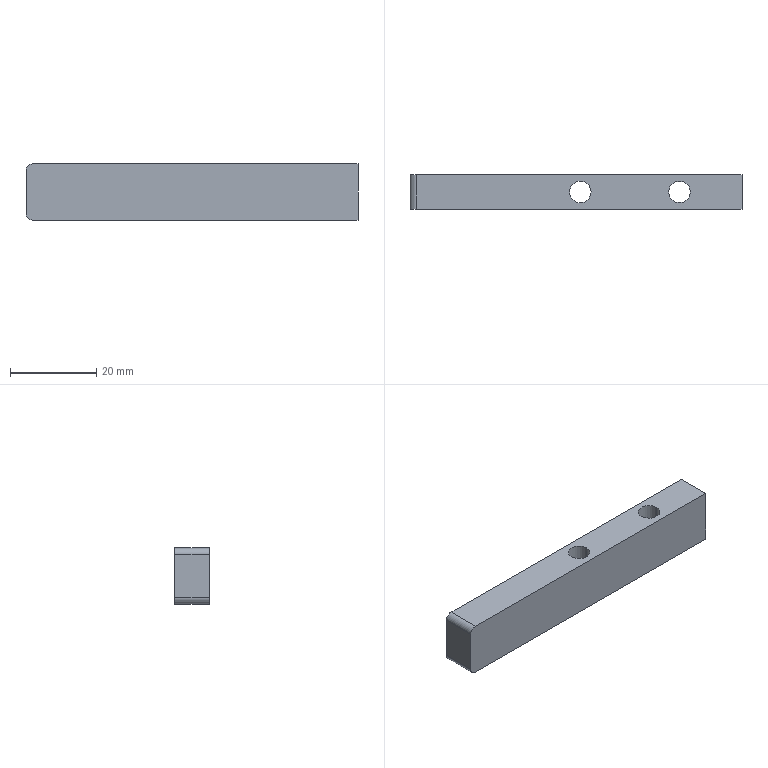Part | 1 solid | 15 faces | box 77 x 8 x 13 mm | volume 6967 mm3 | cylinder 8 | plane 7 | commonest cylinder face diameters 5 x4 3 x2 11 x2
STEP:
#1=CARTESIAN_POINT('',(-14.,4.,-6.5));
#2=VERTEX_POINT('',#1);
#3=CARTESIAN_POINT('',(-9.,4.,-6.5));
#4=VERTEX_POINT('',#3);
#5=CARTESIAN_POINT('',(-11.5,4.,-6.5));
#6=DIRECTION('',(0.,0.,1.));
#7=DIRECTION('',(1.,0.,0.));
#8=AXIS2_PLACEMENT_3D('',#5,#6,#7);
#9=CIRCLE('',#8,2.5);
#10=EDGE_CURVE('',#2,#4,#9,.T.);
#11=ORIENTED_EDGE('',*,*,#10,.F.);
#12=CARTESIAN_POINT('',(-14.,4.,6.5));
#13=VERTEX_POINT('',#12);
#14=CARTESIAN_POINT('',(-14.,4.,-6.5));
#15=DIRECTION('',(0.,0.,1.));
#16=VECTOR('',#15,1000.);
#17=LINE('',#14,#16);
#18=EDGE_CURVE('',#2,#13,#17,.T.);
#19=ORIENTED_EDGE('',*,*,#18,.T.);
#20=CARTESIAN_POINT('',(-9.,4.,6.5));
#21=VERTEX_POINT('',#20);
#22=CARTESIAN_POINT('',(-11.5,4.,6.5));
#23=DIRECTION('',(0.,0.,1.));
#24=DIRECTION('',(1.,0.,0.));
#25=AXIS2_PLACEMENT_3D('',#22,#23,#24);
#26=CIRCLE('',#25,2.5);
#27=EDGE_CURVE('',#13,#21,#26,.T.);
#28=ORIENTED_EDGE('',*,*,#27,.T.);
#29=CARTESIAN_POINT('',(-9.,4.,-6.5));
#30=DIRECTION('',(0.,0.,1.));
#31=VECTOR('',#30,1000.);
#32=LINE('',#29,#31);
#33=EDGE_CURVE('',#4,#21,#32,.T.);
#34=ORIENTED_EDGE('',*,*,#33,.F.);
#35=EDGE_LOOP('',(#11,#19,#28,#34));
#36=FACE_OUTER_BOUND('',#35,.T.);
#37=CARTESIAN_POINT('',(-11.5,4.,-6.5));
#38=DIRECTION('',(0.,0.,1.));
#39=DIRECTION('',(1.,0.,0.));
#40=AXIS2_PLACEMENT_3D('',#37,#38,#39);
#41=CYLINDRICAL_SURFACE('',#40,2.5);
#42=ADVANCED_FACE('',(#36),#41,.F.);
#43=CARTESIAN_POINT('',(9.,4.,-6.5));
#44=VERTEX_POINT('',#43);
#45=CARTESIAN_POINT('',(14.,4.,-6.5));
#46=VERTEX_POINT('',#45);
#47=CARTESIAN_POINT('',(11.5,4.,-6.5));
#48=DIRECTION('',(0.,0.,1.));
#49=DIRECTION('',(1.,0.,0.));
#50=AXIS2_PLACEMENT_3D('',#47,#48,#49);
#51=CIRCLE('',#50,2.5);
#52=EDGE_CURVE('',#44,#46,#51,.T.);
#53=ORIENTED_EDGE('',*,*,#52,.F.);
#54=CARTESIAN_POINT('',(9.,4.,6.5));
#55=VERTEX_POINT('',#54);
#56=CARTESIAN_POINT('',(9.,4.,-6.5));
#57=DIRECTION('',(0.,0.,1.));
#58=VECTOR('',#57,1000.);
#59=LINE('',#56,#58);
#60=EDGE_CURVE('',#44,#55,#59,.T.);
#61=ORIENTED_EDGE('',*,*,#60,.T.);
#62=CARTESIAN_POINT('',(14.,4.,6.5));
#63=VERTEX_POINT('',#62);
#64=CARTESIAN_POINT('',(11.5,4.,6.5));
#65=DIRECTION('',(0.,0.,1.));
#66=DIRECTION('',(1.,0.,0.));
#67=AXIS2_PLACEMENT_3D('',#64,#65,#66);
#68=CIRCLE('',#67,2.5);
#69=EDGE_CURVE('',#55,#63,#68,.T.);
#70=ORIENTED_EDGE('',*,*,#69,.T.);
#71=CARTESIAN_POINT('',(14.,4.,-6.5));
#72=DIRECTION('',(0.,0.,1.));
#73=VECTOR('',#72,1000.);
#74=LINE('',#71,#73);
#75=EDGE_CURVE('',#46,#63,#74,.T.);
#76=ORIENTED_EDGE('',*,*,#75,.F.);
#77=EDGE_LOOP('',(#53,#61,#70,#76));
#78=FACE_OUTER_BOUND('',#77,.T.);
#79=CARTESIAN_POINT('',(11.5,4.,-6.5));
#80=DIRECTION('',(0.,0.,1.));
#81=DIRECTION('',(1.,0.,0.));
#82=AXIS2_PLACEMENT_3D('',#79,#80,#81);
#83=CYLINDRICAL_SURFACE('',#82,2.5);
#84=ADVANCED_FACE('',(#78),#83,.F.);
#85=CARTESIAN_POINT('',(0.,2.5,5.5));
#86=VERTEX_POINT('',#85);
#87=CARTESIAN_POINT('',(0.,2.5,-5.5));
#88=VERTEX_POINT('',#87);
#89=CARTESIAN_POINT('',(0.,2.5,0.));
#90=DIRECTION('',(0.,-1.,0.));
#91=DIRECTION('',(0.,0.,-1.));
#92=AXIS2_PLACEMENT_3D('',#89,#90,#91);
#93=CIRCLE('',#92,5.5);
#94=EDGE_CURVE('',#86,#88,#93,.T.);
#95=ORIENTED_EDGE('',*,*,#94,.T.);
#96=CARTESIAN_POINT('',(0.,8.,-5.5));
#97=VERTEX_POINT('',#96);
#98=CARTESIAN_POINT('',(0.,2.5,-5.5));
#99=DIRECTION('',(0.,1.,0.));
#100=VECTOR('',#99,1000.);
#101=LINE('',#98,#100);
#102=EDGE_CURVE('',#88,#97,#101,.T.);
#103=ORIENTED_EDGE('',*,*,#102,.T.);
#104=CARTESIAN_POINT('',(0.,8.,5.5));
#105=VERTEX_POINT('',#104);
#106=CARTESIAN_POINT('',(0.,8.,0.));
#107=DIRECTION('',(0.,-1.,0.));
#108=DIRECTION('',(0.,0.,-1.));
#109=AXIS2_PLACEMENT_3D('',#106,#107,#108);
#110=CIRCLE('',#109,5.5);
#111=EDGE_CURVE('',#105,#97,#110,.T.);
#112=ORIENTED_EDGE('',*,*,#111,.F.);
#113=CARTESIAN_POINT('',(0.,2.5,5.5));
#114=DIRECTION('',(0.,1.,0.));
#115=VECTOR('',#114,1000.);
#116=LINE('',#113,#115);
#117=EDGE_CURVE('',#86,#105,#116,.T.);
#118=ORIENTED_EDGE('',*,*,#117,.F.);
#119=EDGE_LOOP('',(#95,#103,#112,#118));
#120=FACE_OUTER_BOUND('',#119,.T.);
#121=CARTESIAN_POINT('',(0.,2.5,0.));
#122=DIRECTION('',(0.,1.,0.));
#123=DIRECTION('',(0.,0.,1.));
#124=AXIS2_PLACEMENT_3D('',#121,#122,#123);
#125=CYLINDRICAL_SURFACE('',#124,5.5);
#126=ADVANCED_FACE('',(#120),#125,.F.);
#127=CARTESIAN_POINT('',(26.,0.,6.5));
#128=VERTEX_POINT('',#127);
#129=CARTESIAN_POINT('',(26.,0.,-6.5));
#130=VERTEX_POINT('',#129);
#131=CARTESIAN_POINT('',(26.,0.,6.5));
#132=DIRECTION('',(0.,0.,-1.));
#133=VECTOR('',#132,1000.);
#134=LINE('',#131,#133);
#135=EDGE_CURVE('',#128,#130,#134,.T.);
#136=ORIENTED_EDGE('',*,*,#135,.T.);
#137=CARTESIAN_POINT('',(26.,8.,-6.5));
#138=VERTEX_POINT('',#137);
#139=CARTESIAN_POINT('',(26.,8.,-6.5));
#140=DIRECTION('',(0.,-1.,0.));
#141=VECTOR('',#140,1000.);
#142=LINE('',#139,#141);
#143=EDGE_CURVE('',#138,#130,#142,.T.);
#144=ORIENTED_EDGE('',*,*,#143,.F.);
#145=CARTESIAN_POINT('',(26.,8.,6.5));
#146=VERTEX_POINT('',#145);
#147=CARTESIAN_POINT('',(26.,8.,6.5));
#148=DIRECTION('',(0.,0.,-1.));
#149=VECTOR('',#148,1000.);
#150=LINE('',#147,#149);
#151=EDGE_CURVE('',#146,#138,#150,.T.);
#152=ORIENTED_EDGE('',*,*,#151,.F.);
#153=CARTESIAN_POINT('',(26.,8.,6.5));
#154=DIRECTION('',(0.,-1.,0.));
#155=VECTOR('',#154,1000.);
#156=LINE('',#153,#155);
#157=EDGE_CURVE('',#146,#128,#156,.T.);
#158=ORIENTED_EDGE('',*,*,#157,.T.);
#159=EDGE_LOOP('',(#136,#144,#152,#158));
#160=FACE_OUTER_BOUND('',#159,.T.);
#161=CARTESIAN_POINT('',(26.,8.,6.5));
#162=DIRECTION('',(-1.,0.,0.));
#163=DIRECTION('',(0.,0.,1.));
#164=AXIS2_PLACEMENT_3D('',#161,#162,#163);
#165=PLANE('',#164);
#166=ADVANCED_FACE('',(#160),#165,.F.);
#167=CARTESIAN_POINT('',(-11.5,4.,-6.5));
#168=DIRECTION('',(0.,0.,1.));
#169=DIRECTION('',(1.,0.,0.));
#170=AXIS2_PLACEMENT_3D('',#167,#168,#169);
#171=CIRCLE('',#170,2.5);
#172=EDGE_CURVE('',#4,#2,#171,.T.);
#173=ORIENTED_EDGE('',*,*,#172,.T.);
#174=ORIENTED_EDGE('',*,*,#10,.T.);
#175=EDGE_LOOP('',(#173,#174));
#176=FACE_BOUND('',#175,.T.);
#177=CARTESIAN_POINT('',(11.5,4.,-6.5));
#178=DIRECTION('',(0.,0.,1.));
#179=DIRECTION('',(1.,0.,0.));
#180=AXIS2_PLACEMENT_3D('',#177,#178,#179);
#181=CIRCLE('',#180,2.5);
#182=EDGE_CURVE('',#46,#44,#181,.T.);
#183=ORIENTED_EDGE('',*,*,#182,.T.);
#184=ORIENTED_EDGE('',*,*,#52,.T.);
#185=EDGE_LOOP('',(#183,#184));
#186=FACE_BOUND('',#185,.T.);
#187=CARTESIAN_POINT('',(-49.5,0.,-6.5));
#188=VERTEX_POINT('',#187);
#189=CARTESIAN_POINT('',(-16.,0.,-6.5));
#190=DIRECTION('',(-1.,0.,0.));
#191=VECTOR('',#190,1000.);
#192=LINE('',#189,#191);
#193=EDGE_CURVE('',#130,#188,#192,.T.);
#194=ORIENTED_EDGE('',*,*,#193,.T.);
#195=CARTESIAN_POINT('',(-49.5,8.,-6.5));
#196=VERTEX_POINT('',#195);
#197=CARTESIAN_POINT('',(-49.5,8.,-6.5));
#198=DIRECTION('',(0.,1.,0.));
#199=VECTOR('',#198,1000.);
#200=LINE('',#197,#199);
#201=EDGE_CURVE('',#188,#196,#200,.T.);
#202=ORIENTED_EDGE('',*,*,#201,.T.);
#203=CARTESIAN_POINT('',(-16.,8.,-6.5));
#204=DIRECTION('',(-1.,0.,0.));
#205=VECTOR('',#204,1000.);
#206=LINE('',#203,#205);
#207=EDGE_CURVE('',#138,#196,#206,.T.);
#208=ORIENTED_EDGE('',*,*,#207,.F.);
#209=ORIENTED_EDGE('',*,*,#143,.T.);
#210=EDGE_LOOP('',(#194,#202,#208,#209));
#211=FACE_OUTER_BOUND('',#210,.T.);
#212=CARTESIAN_POINT('',(-16.,8.,-6.5));
#213=DIRECTION('',(0.,0.,1.));
#214=DIRECTION('',(1.,0.,0.));
#215=AXIS2_PLACEMENT_3D('',#212,#213,#214);
#216=PLANE('',#215);
#217=ADVANCED_FACE('',(#176,#186,#211),#216,.F.);
#218=CARTESIAN_POINT('',(-51.,0.,-5.));
#219=VERTEX_POINT('',#218);
#220=CARTESIAN_POINT('',(-51.,0.,5.));
#221=VERTEX_POINT('',#220);
#222=CARTESIAN_POINT('',(-51.,0.,6.5));
#223=DIRECTION('',(0.,0.,1.));
#224=VECTOR('',#223,1000.);
#225=LINE('',#222,#224);
#226=EDGE_CURVE('',#219,#221,#225,.T.);
#227=ORIENTED_EDGE('',*,*,#226,.T.);
#228=CARTESIAN_POINT('',(-51.,8.,5.));
#229=VERTEX_POINT('',#228);
#230=CARTESIAN_POINT('',(-51.,8.,5.));
#231=DIRECTION('',(0.,1.,0.));
#232=VECTOR('',#231,1000.);
#233=LINE('',#230,#232);
#234=EDGE_CURVE('',#221,#229,#233,.T.);
#235=ORIENTED_EDGE('',*,*,#234,.T.);
#236=CARTESIAN_POINT('',(-51.,8.,-5.));
#237=VERTEX_POINT('',#236);
#238=CARTESIAN_POINT('',(-51.,8.,6.5));
#239=DIRECTION('',(0.,0.,1.));
#240=VECTOR('',#239,1000.);
#241=LINE('',#238,#240);
#242=EDGE_CURVE('',#237,#229,#241,.T.);
#243=ORIENTED_EDGE('',*,*,#242,.F.);
#244=CARTESIAN_POINT('',(-51.,8.,-5.));
#245=DIRECTION('',(0.,-1.,0.));
#246=VECTOR('',#245,1000.);
#247=LINE('',#244,#246);
#248=EDGE_CURVE('',#237,#219,#247,.T.);
#249=ORIENTED_EDGE('',*,*,#248,.T.);
#250=EDGE_LOOP('',(#227,#235,#243,#249));
#251=FACE_OUTER_BOUND('',#250,.T.);
#252=CARTESIAN_POINT('',(-51.,8.,6.5));
#253=DIRECTION('',(1.,0.,0.));
#254=DIRECTION('',(0.,0.,-1.));
#255=AXIS2_PLACEMENT_3D('',#252,#253,#254);
#256=PLANE('',#255);
#257=ADVANCED_FACE('',(#251),#256,.F.);
#258=CARTESIAN_POINT('',(-11.5,4.,6.5));
#259=DIRECTION('',(0.,0.,1.));
#260=DIRECTION('',(1.,0.,0.));
#261=AXIS2_PLACEMENT_3D('',#258,#259,#260);
#262=CIRCLE('',#261,2.5);
#263=EDGE_CURVE('',#21,#13,#262,.T.);
#264=ORIENTED_EDGE('',*,*,#263,.F.);
#265=ORIENTED_EDGE('',*,*,#27,.F.);
#266=EDGE_LOOP('',(#264,#265));
#267=FACE_BOUND('',#266,.T.);
#268=CARTESIAN_POINT('',(11.5,4.,6.5));
#269=DIRECTION('',(0.,0.,1.));
#270=DIRECTION('',(1.,0.,0.));
#271=AXIS2_PLACEMENT_3D('',#268,#269,#270);
#272=CIRCLE('',#271,2.5);
#273=EDGE_CURVE('',#63,#55,#272,.T.);
#274=ORIENTED_EDGE('',*,*,#273,.F.);
#275=ORIENTED_EDGE('',*,*,#69,.F.);
#276=EDGE_LOOP('',(#274,#275));
#277=FACE_BOUND('',#276,.T.);
#278=CARTESIAN_POINT('',(-49.5,8.,6.5));
#279=VERTEX_POINT('',#278);
#280=CARTESIAN_POINT('',(-16.,8.,6.5));
#281=DIRECTION('',(1.,0.,0.));
#282=VECTOR('',#281,1000.);
#283=LINE('',#280,#282);
#284=EDGE_CURVE('',#279,#146,#283,.T.);
#285=ORIENTED_EDGE('',*,*,#284,.F.);
#286=CARTESIAN_POINT('',(-49.5,0.,6.5));
#287=VERTEX_POINT('',#286);
#288=CARTESIAN_POINT('',(-49.5,8.,6.5));
#289=DIRECTION('',(0.,-1.,0.));
#290=VECTOR('',#289,1000.);
#291=LINE('',#288,#290);
#292=EDGE_CURVE('',#279,#287,#291,.T.);
#293=ORIENTED_EDGE('',*,*,#292,.T.);
#294=CARTESIAN_POINT('',(-16.,0.,6.5));
#295=DIRECTION('',(1.,0.,0.));
#296=VECTOR('',#295,1000.);
#297=LINE('',#294,#296);
#298=EDGE_CURVE('',#287,#128,#297,.T.);
#299=ORIENTED_EDGE('',*,*,#298,.T.);
#300=ORIENTED_EDGE('',*,*,#157,.F.);
#301=EDGE_LOOP('',(#285,#293,#299,#300));
#302=FACE_OUTER_BOUND('',#301,.T.);
#303=CARTESIAN_POINT('',(-16.,8.,6.5));
#304=DIRECTION('',(0.,0.,-1.));
#305=DIRECTION('',(-1.,0.,0.));
#306=AXIS2_PLACEMENT_3D('',#303,#304,#305);
#307=PLANE('',#306);
#308=ADVANCED_FACE('',(#267,#277,#302),#307,.F.);
#309=ORIENTED_EDGE('',*,*,#111,.T.);
#310=CARTESIAN_POINT('',(0.,8.,0.));
#311=DIRECTION('',(0.,-1.,0.));
#312=DIRECTION('',(0.,0.,-1.));
#313=AXIS2_PLACEMENT_3D('',#310,#311,#312);
#314=CIRCLE('',#313,5.5);
#315=EDGE_CURVE('',#97,#105,#314,.T.);
#316=ORIENTED_EDGE('',*,*,#315,.T.);
#317=EDGE_LOOP('',(#309,#316));
#318=FACE_BOUND('',#317,.T.);
#319=ORIENTED_EDGE('',*,*,#242,.T.);
#320=CARTESIAN_POINT('',(-49.5,8.,5.));
#321=DIRECTION('',(0.,1.,0.));
#322=DIRECTION('',(0.,0.,-1.));
#323=AXIS2_PLACEMENT_3D('',#320,#321,#322);
#324=CIRCLE('',#323,1.5);
#325=EDGE_CURVE('',#229,#279,#324,.T.);
#326=ORIENTED_EDGE('',*,*,#325,.T.);
#327=ORIENTED_EDGE('',*,*,#284,.T.);
#328=ORIENTED_EDGE('',*,*,#151,.T.);
#329=ORIENTED_EDGE('',*,*,#207,.T.);
#330=CARTESIAN_POINT('',(-49.5,8.,-5.));
#331=DIRECTION('',(0.,1.,0.));
#332=DIRECTION('',(0.,0.,-1.));
#333=AXIS2_PLACEMENT_3D('',#330,#331,#332);
#334=CIRCLE('',#333,1.5);
#335=EDGE_CURVE('',#196,#237,#334,.T.);
#336=ORIENTED_EDGE('',*,*,#335,.T.);
#337=EDGE_LOOP('',(#319,#326,#327,#328,#329,#336));
#338=FACE_OUTER_BOUND('',#337,.T.);
#339=CARTESIAN_POINT('',(0.,8.,0.));
#340=DIRECTION('',(0.,-1.,0.));
#341=DIRECTION('',(0.,0.,-1.));
#342=AXIS2_PLACEMENT_3D('',#339,#340,#341);
#343=PLANE('',#342);
#344=ADVANCED_FACE('',(#318,#338),#343,.F.);
#345=ORIENTED_EDGE('',*,*,#298,.F.);
#346=CARTESIAN_POINT('',(-49.5,0.,5.));
#347=DIRECTION('',(0.,-1.,0.));
#348=DIRECTION('',(0.,0.,-1.));
#349=AXIS2_PLACEMENT_3D('',#346,#347,#348);
#350=CIRCLE('',#349,1.5);
#351=EDGE_CURVE('',#287,#221,#350,.T.);
#352=ORIENTED_EDGE('',*,*,#351,.T.);
#353=ORIENTED_EDGE('',*,*,#226,.F.);
#354=CARTESIAN_POINT('',(-49.5,0.,-5.));
#355=DIRECTION('',(0.,-1.,0.));
#356=DIRECTION('',(0.,0.,-1.));
#357=AXIS2_PLACEMENT_3D('',#354,#355,#356);
#358=CIRCLE('',#357,1.5);
#359=EDGE_CURVE('',#219,#188,#358,.T.);
#360=ORIENTED_EDGE('',*,*,#359,.T.);
#361=ORIENTED_EDGE('',*,*,#193,.F.);
#362=ORIENTED_EDGE('',*,*,#135,.F.);
#363=EDGE_LOOP('',(#345,#352,#353,#360,#361,#362));
#364=FACE_OUTER_BOUND('',#363,.T.);
#365=CARTESIAN_POINT('',(0.,0.,0.));
#366=DIRECTION('',(0.,-1.,0.));
#367=DIRECTION('',(0.,0.,-1.));
#368=AXIS2_PLACEMENT_3D('',#365,#366,#367);
#369=PLANE('',#368);
#370=ADVANCED_FACE('',(#364),#369,.T.);
#371=ORIENTED_EDGE('',*,*,#102,.F.);
#372=CARTESIAN_POINT('',(0.,2.5,0.));
#373=DIRECTION('',(0.,-1.,0.));
#374=DIRECTION('',(0.,0.,-1.));
#375=AXIS2_PLACEMENT_3D('',#372,#373,#374);
#376=CIRCLE('',#375,5.5);
#377=EDGE_CURVE('',#88,#86,#376,.T.);
#378=ORIENTED_EDGE('',*,*,#377,.T.);
#379=ORIENTED_EDGE('',*,*,#117,.T.);
#380=ORIENTED_EDGE('',*,*,#315,.F.);
#381=EDGE_LOOP('',(#371,#378,#379,#380));
#382=FACE_OUTER_BOUND('',#381,.T.);
#383=CARTESIAN_POINT('',(0.,2.5,0.));
#384=DIRECTION('',(0.,1.,0.));
#385=DIRECTION('',(0.,0.,1.));
#386=AXIS2_PLACEMENT_3D('',#383,#384,#385);
#387=CYLINDRICAL_SURFACE('',#386,5.5);
#388=ADVANCED_FACE('',(#382),#387,.F.);
#389=ORIENTED_EDGE('',*,*,#94,.F.);
#390=ORIENTED_EDGE('',*,*,#377,.F.);
#391=EDGE_LOOP('',(#389,#390));
#392=FACE_OUTER_BOUND('',#391,.T.);
#393=CARTESIAN_POINT('',(0.,2.5,0.));
#394=DIRECTION('',(0.,-1.,0.));
#395=DIRECTION('',(0.,0.,-1.));
#396=AXIS2_PLACEMENT_3D('',#393,#394,#395);
#397=PLANE('',#396);
#398=ADVANCED_FACE('',(#392),#397,.F.);
#399=ORIENTED_EDGE('',*,*,#60,.F.);
#400=ORIENTED_EDGE('',*,*,#182,.F.);
#401=ORIENTED_EDGE('',*,*,#75,.T.);
#402=ORIENTED_EDGE('',*,*,#273,.T.);
#403=EDGE_LOOP('',(#399,#400,#401,#402));
#404=FACE_OUTER_BOUND('',#403,.T.);
#405=CARTESIAN_POINT('',(11.5,4.,-6.5));
#406=DIRECTION('',(0.,0.,1.));
#407=DIRECTION('',(1.,0.,0.));
#408=AXIS2_PLACEMENT_3D('',#405,#406,#407);
#409=CYLINDRICAL_SURFACE('',#408,2.5);
#410=ADVANCED_FACE('',(#404),#409,.F.);
#411=ORIENTED_EDGE('',*,*,#18,.F.);
#412=ORIENTED_EDGE('',*,*,#172,.F.);
#413=ORIENTED_EDGE('',*,*,#33,.T.);
#414=ORIENTED_EDGE('',*,*,#263,.T.);
#415=EDGE_LOOP('',(#411,#412,#413,#414));
#416=FACE_OUTER_BOUND('',#415,.T.);
#417=CARTESIAN_POINT('',(-11.5,4.,-6.5));
#418=DIRECTION('',(0.,0.,1.));
#419=DIRECTION('',(1.,0.,0.));
#420=AXIS2_PLACEMENT_3D('',#417,#418,#419);
#421=CYLINDRICAL_SURFACE('',#420,2.5);
#422=ADVANCED_FACE('',(#416),#421,.F.);
#423=ORIENTED_EDGE('',*,*,#325,.F.);
#424=ORIENTED_EDGE('',*,*,#234,.F.);
#425=ORIENTED_EDGE('',*,*,#351,.F.);
#426=ORIENTED_EDGE('',*,*,#292,.F.);
#427=EDGE_LOOP('',(#423,#424,#425,#426));
#428=FACE_OUTER_BOUND('',#427,.T.);
#429=CARTESIAN_POINT('',(-49.5,8.,5.));
#430=DIRECTION('',(0.,-1.,0.));
#431=DIRECTION('',(0.,0.,-1.));
#432=AXIS2_PLACEMENT_3D('',#429,#430,#431);
#433=CYLINDRICAL_SURFACE('',#432,1.5);
#434=ADVANCED_FACE('',(#428),#433,.T.);
#435=ORIENTED_EDGE('',*,*,#335,.F.);
#436=ORIENTED_EDGE('',*,*,#201,.F.);
#437=ORIENTED_EDGE('',*,*,#359,.F.);
#438=ORIENTED_EDGE('',*,*,#248,.F.);
#439=EDGE_LOOP('',(#435,#436,#437,#438));
#440=FACE_OUTER_BOUND('',#439,.T.);
#441=CARTESIAN_POINT('',(-49.5,8.,-5.));
#442=DIRECTION('',(0.,-1.,0.));
#443=DIRECTION('',(0.,0.,-1.));
#444=AXIS2_PLACEMENT_3D('',#441,#442,#443);
#445=CYLINDRICAL_SURFACE('',#444,1.5);
#446=ADVANCED_FACE('',(#440),#445,.T.);
#447=CLOSED_SHELL('',(#42,#84,#126,#166,#217,#257,#308,#344,#370,#388,#398,#410,#422,#434,#446));
#448=MANIFOLD_SOLID_BREP('',#447);
#449=CARTESIAN_POINT('',(0.,0.,0.));
#450=DIRECTION('',(0.,0.,1.));
#451=DIRECTION('',(1.,0.,0.));
#452=AXIS2_PLACEMENT_3D('',#449,#450,#451);
#453=(LENGTH_UNIT()NAMED_UNIT(*)SI_UNIT(.MILLI.,.METRE.));
#454=UNCERTAINTY_MEASURE_WITH_UNIT(LENGTH_MEASURE(0.00001),#453,'','');
#455=(NAMED_UNIT(*)PLANE_ANGLE_UNIT()SI_UNIT($,.RADIAN.));
#456=(NAMED_UNIT(*)SI_UNIT($,.STERADIAN.)SOLID_ANGLE_UNIT());
#457=(GEOMETRIC_REPRESENTATION_CONTEXT(3)GLOBAL_UNCERTAINTY_ASSIGNED_CONTEXT((#454))GLOBAL_UNIT_ASSIGNED_CONTEXT((#453,#455,#456))REPRESENTATION_CONTEXT('',''));
#458=ADVANCED_BREP_SHAPE_REPRESENTATION('',(#448,#452),#457);